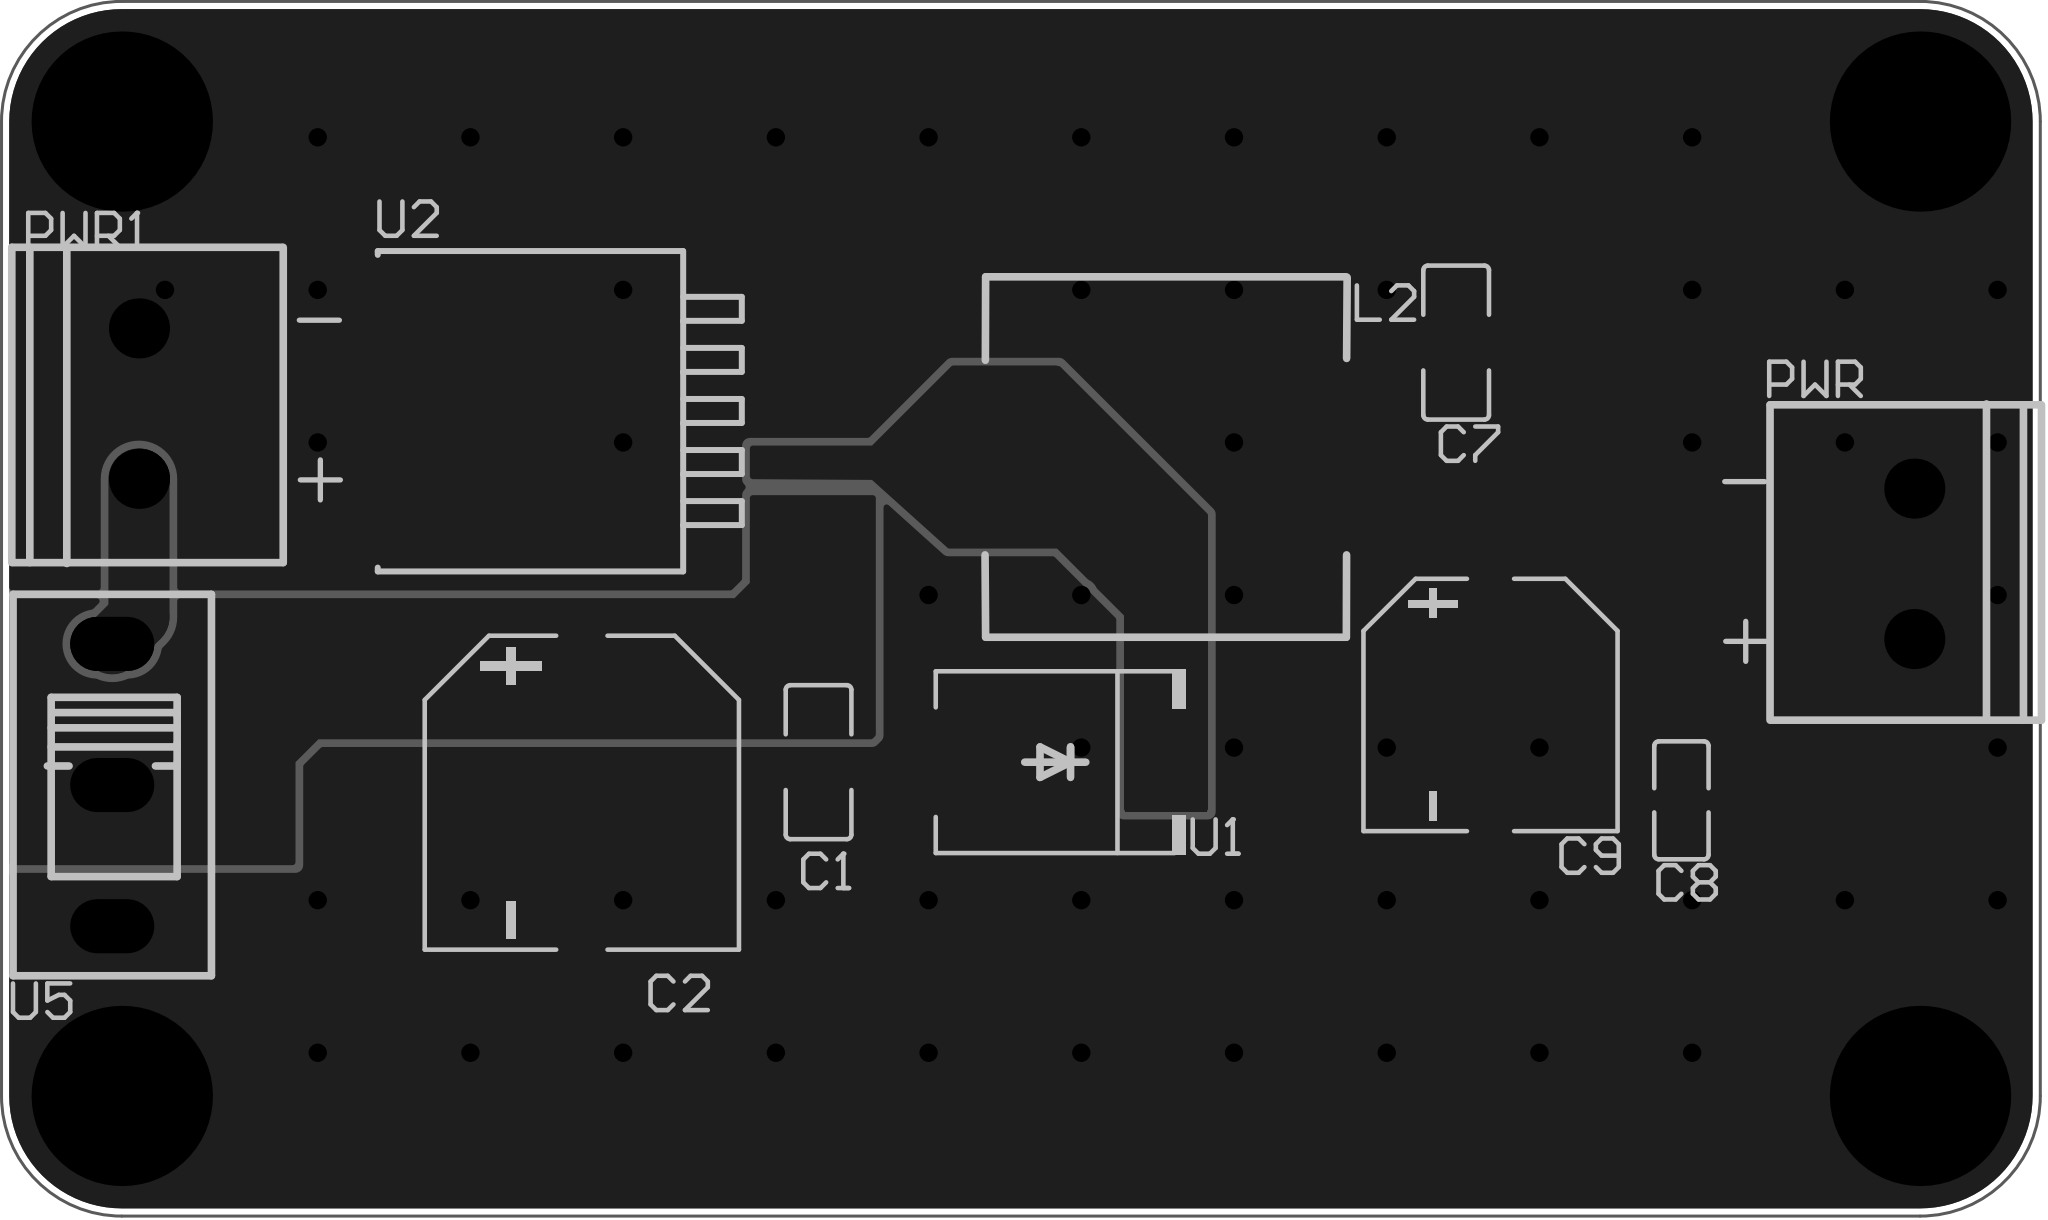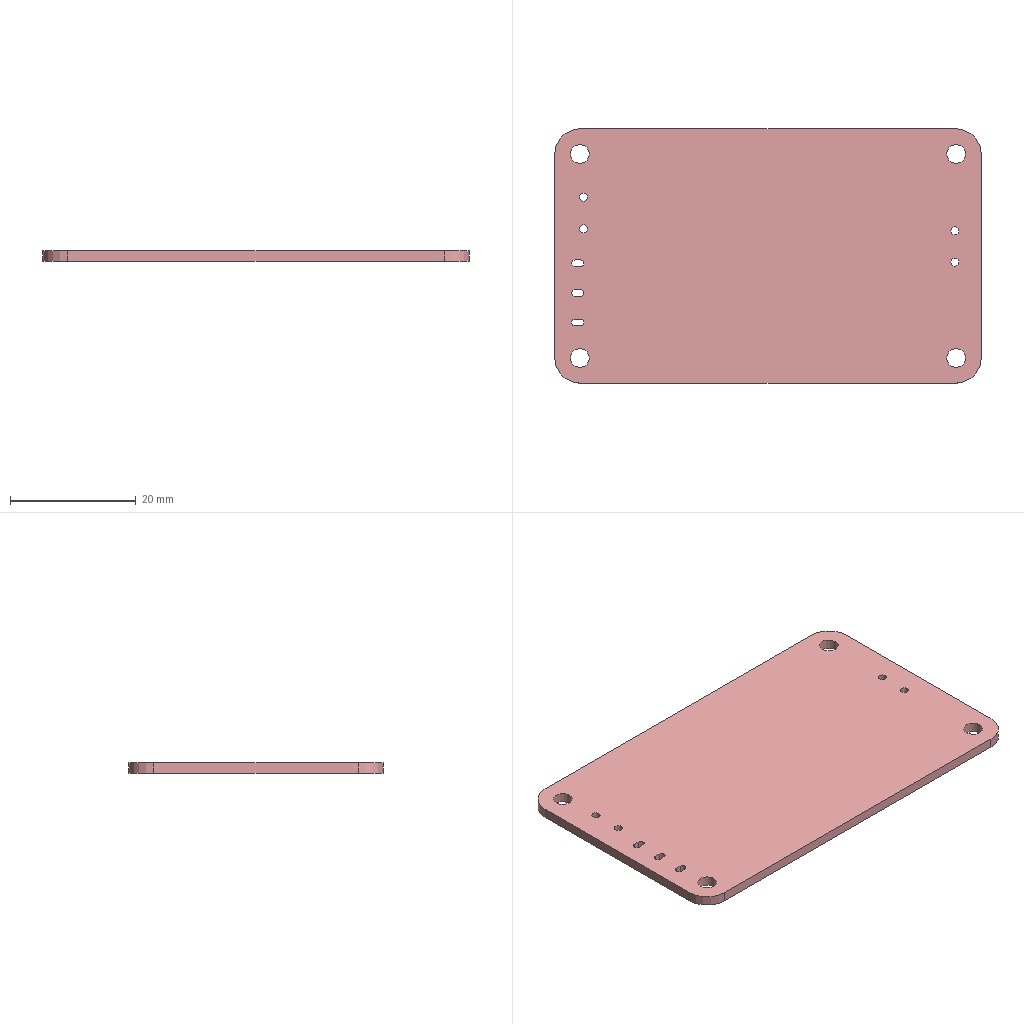Circuit board layout | Altium Designer | box 67.8 x 40.4 x 1.6 mm
Layer stack:
# Altium Designer layer stack of  (unit mm; dielectric type: 0 none, 1 core, 2 prepreg, 3 surface material)
index,name,kind,layer,copper_thickness_mm,dielectric_type,dielectric_thickness_mm,dielectric_material,dielectric_constant
0,Top Paste Mask Layer,other,,,,,,
1,Top Silkscreen Layer,other,,,,,,
2,Top Solder Mask Layer,dielectric,,,3,0.01,,3.3
3,Top Layer,copper,Top Layer,0.035,,,,
4,Dielectric1,dielectric,,,3,1.51,FR4,4.5
5,Bottom Layer,copper,Bottom Layer,0.035,,,,
6,Bottom Solder Mask Layer,dielectric,,,3,0.01,,3.3
7,Bottom Silkscreen Layer,other,,,,,,
8,Bottom Paste Mask Layer,other,,,,,,
# drill layer pairs: low layer,high layer
drill_pair,Top Layer,Bottom Layer
Part placement:
Designator,Comment,Layer,Footprint,Center-X(mm),Center-Y(mm),Rotation
U2,LM2596HVS-12.0,TopLayer,TO-263-5_L10.0-W8.4-P1.70-LS15.3-BR,106.007,117.856,0
C9,220uF,TopLayer,CAP-SMD_BD8.0-L8.3-W8.3-FD-1,134.112,108.077,270
U1,SS56,TopLayer,SMC_L6.9-W5.9-LS7.9-RD,119.634,106.172,180
PWR,CONN-TH_2P-P5.00,TopLayer,CONN-TH_2P-P5.00,148.209,112.776,270
PWR1,CONN-TH_2P-P5.00,TopLayer,CONN-TH_2P-P5.00,89.154,118.11,90
C2,220uF,TopLayer,CAP-SMD_BD10.0-L10.3-W10.3-FD-LS11.3,103.886,105.156,270
L2,68uH,TopLayer,IND-SMD_L12.0-W12.0_744771008,123.317,116.332,0
C7,100nF,TopLayer,C1206,132.969,120.142,270
C8,10uF,TopLayer,C0805,140.462,104.902,90
U5,SS-12D10-G5,TopLayer,SW-TH_SS-12D10-G050,88.265,105.41,270
C1,100nF,TopLayer,C1206,111.76,106.172,90
Pad and via stacks:
# Altium Designer via and pad stacks of  (unit mm). Each distinct definition once, with the count of objects using it.
# via: kind,start_layer,end_layer,hole_mm,diameter_mm,mode(0 simple;1 top-mid-bottom;2 full stack),diameter_per_layer,count,example_net
# pad: kind,layer,hole_mm,hole_type(0 round;1 square;2 slot),plating,top_size,top_shape(1 round;2 rect;3 octagon;9 rounded rect),mid_size,bottom_size,mode,footprint,size_per_layer,count,example
pad,Multi-Layer,3,0,plated,6x6,1,6x6,6x6,0,,,4,1
pad,Multi-Layer,1.3,0,plated,2x2,1,2x2,2x2,0,CONN-TH_2P-P5.00,,4,PWR.1
pad,Multi-Layer,1.1,2,plated,1.8x2.8,1,1.8x2.8,1.8x2.8,0,SW-TH_SS-12D10-G050,,3,U5.1
pad,Top Layer,0,0,plated,4x1.02,2,4x1.02,4x1.02,0,TO-263-5_L10.0-W8.4-P1.70-LS15.3-BR,,5,U2.1
pad,Top Layer,0,0,plated,8.4x10,2,8.4x10,8.4x10,0,TO-263-5_L10.0-W8.4-P1.70-LS15.3-BR,,1,U2.6
pad,Top Layer,0,0,plated,3.61x1.26,2,3.61x1.26,3.61x1.26,0,CAP-SMD_BD8.0-L8.3-W8.3-FD-1,,2,C9.1
pad,Top Layer,0,0,plated,2.7x3.3,2,2.7x3.3,2.7x3.3,0,SMC_L6.9-W5.9-LS7.9-RD,,2,U1.2
pad,Top Layer,0,0,plated,4.5x1.65,2,4.5x1.65,4.5x1.65,0,CAP-SMD_BD10.0-L10.3-W10.3-FD-LS11.3,,2,C2.1
pad,Top Layer,0,0,plated,3.5x6,2,3.5x6,3.5x6,0,IND-SMD_L12.0-W12.0_744771008,,2,L2.1
pad,Top Layer,0,0,plated,1.485x1.728,2,1.485x1.728,1.485x1.728,0,C1206,,4,C7.2
pad,Top Layer,0,0,plated,1.41x1.35,2,1.41x1.35,1.41x1.35,0,C0805,,2,C8.2
via,Top Layer,Bottom Layer,0.3048,0.61,0,,56,GND
Copper pours:
name,layer,net,type(0 solid;1 hatched;2 none)
Top Layer-VCC,Top Layer,VCC,0
Top Layer-$1N2845,Top Layer,$1N2845,0
Top Layer-$1N2845 1,Top Layer,$1N2845,0
Top Layer-GND,Top Layer,GND,0
Top Layer-+12V,Top Layer,+12V,0
Bottom Layer-GND,Bottom Layer,GND,0
Design rules, without the lines most boards share:
# Altium Designer design rules of  (exported by Altium Designer, unit mm)
# columns: name | kind | enabled | priority | scope1 | scope2 | descriptor | typed fields (field=value)
Plane_innerPlane | 0 | disabled | 1 | All | All | Clearance Constraint (Gap=6mil) (Disabled)(All),(All) | gap=0.1524
Plane_innerPlane_1 | 63 | disabled | 1 | All | All | Board Clearance Constraint (Gap=0mil) (Disabled)(All) |
Copper_copperRegion | 0 | disabled | 2 | All | All | Clearance Constraint (Gap=6mil) (Disabled)(All),(All) | gap=0.1524
Copper_copperRegion_1 | 63 | disabled | 2 | All | All | Board Clearance Constraint (Gap=0mil) (Disabled)(All) |
safeClearance | 0 | enabled | 3 | All | All | Clearance Constraint (Gap=6mil) (All),(All) | gap=0.1524
safeClearance_1 | 63 | enabled | 3 | All | All | Board Clearance Constraint (Gap=0mil) (All) |
otherClearance | 52 | enabled | 1 | All | All | Hole To Hole Clearance (Gap=11.8mil) (All),(All) | gap=0.2997
trackWidth | 2 | enabled | 1 | All | All | Width Constraint (Min=5mil) (Max=100mil) (Preferred=10mil) (All) |
viaSize | 11 | enabled | 1 | All | All | Routing Via (MinHoleWidth=11.811mil) (MaxHoleWidth=236.22mil) (PreferredHoleWidth=12.008mil) (MinWidth=19.685mil) (MaxWidth=393.701mil) (PreferedWidth=24.016mil) (All) | via_min_hole=0.3 via_max_hole=6 via_preferred_diameter=0.61 via_preferred_hole=0.305
copperRegion | 20 | enabled | 1 | All | All | Polygon Connect Rule(Direct Connect )(Conductor Width=10mil) (Relief Angle=90 Angle) (Entries=4) (Air Gap Width=10mil) (All),(All) | connect_style(0=relief,1=direct,2=none)=1 relief_conductor_width=0.254 relief_entries=4